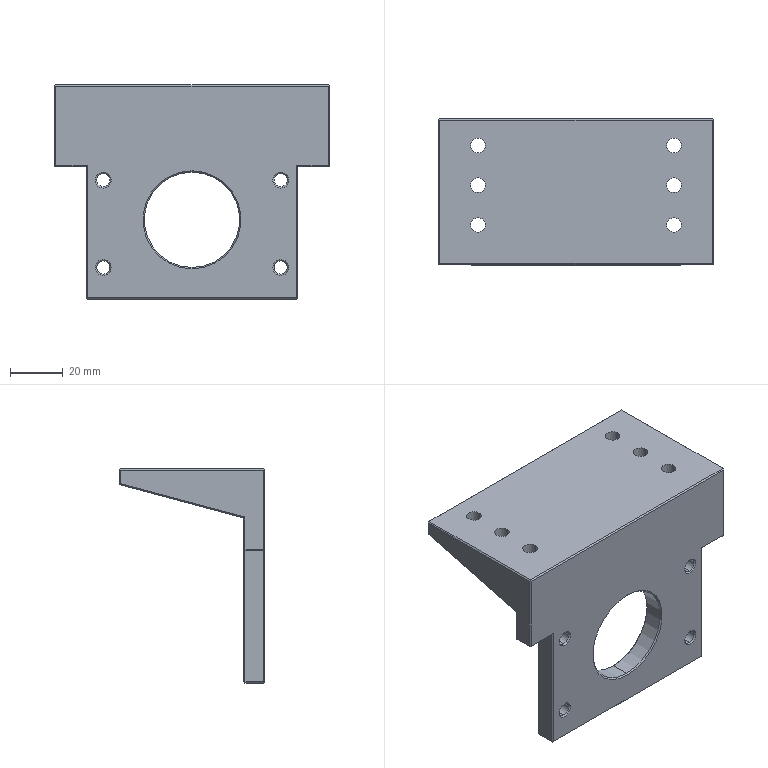Part | STEP file | 1003 | 1 solid | 89 faces | box 104 x 55 x 81 mm | volume 80858 mm3 | plane 47 | cylinder 22 | cone 20 | commonest cylinder face diameters 5.5 x12 5 x8 36 x2